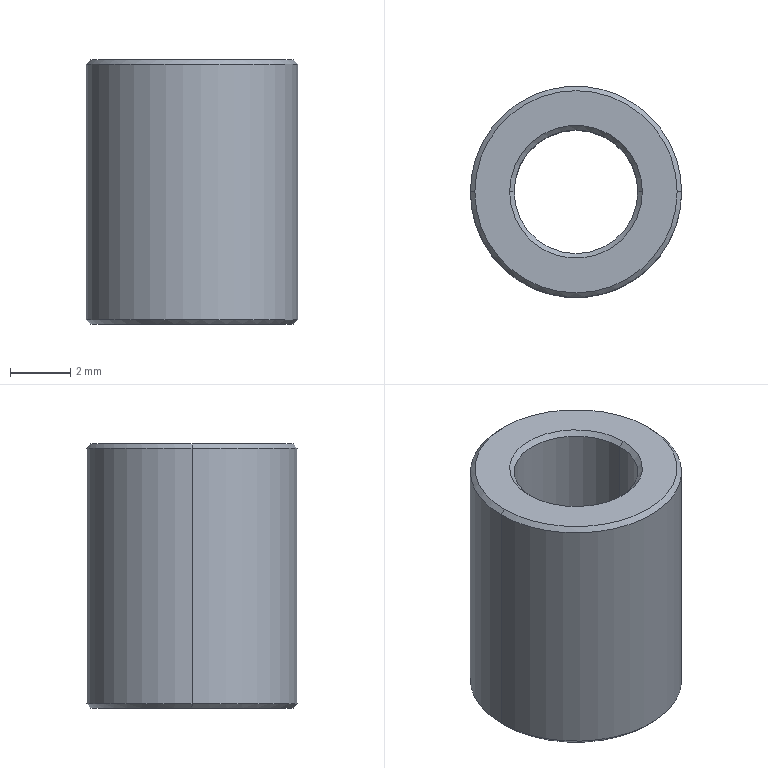Part | NX | features BREP 1 | 1 solid | 14 faces | box 7 x 7 x 8.75 mm | volume 220.433 mm3 | cone 8 | cylinder 4 | plane 2 | commonest cylinder face diameters 4.1 x2 7 x2
STEP:
#1=CARTESIAN_POINT('',(3.35,0.,8.75));
#2=VERTEX_POINT('',#1);
#3=CARTESIAN_POINT('',(3.5,0.,8.6));
#4=VERTEX_POINT('',#3);
#5=CARTESIAN_POINT('',(3.35,0.,8.75));
#6=DIRECTION('',(0.7071,0.,-0.7071));
#7=VECTOR('',#6,1000.);
#8=LINE('',#5,#7);
#9=EDGE_CURVE('',#2,#4,#8,.T.);
#10=ORIENTED_EDGE('',*,*,#9,.F.);
#11=CARTESIAN_POINT('',(-3.35,0.,8.75));
#12=VERTEX_POINT('',#11);
#13=CARTESIAN_POINT('',(0.,0.,8.75));
#14=DIRECTION('',(0.,0.,1.));
#15=DIRECTION('',(1.,0.,0.));
#16=AXIS2_PLACEMENT_3D('',#13,#14,#15);
#17=CIRCLE('',#16,3.35);
#18=EDGE_CURVE('',#12,#2,#17,.T.);
#19=ORIENTED_EDGE('',*,*,#18,.F.);
#20=CARTESIAN_POINT('',(-3.5,0.,8.6));
#21=VERTEX_POINT('',#20);
#22=CARTESIAN_POINT('',(-3.35,0.,8.75));
#23=DIRECTION('',(-0.7071,0.,-0.7071));
#24=VECTOR('',#23,1000.);
#25=LINE('',#22,#24);
#26=EDGE_CURVE('',#12,#21,#25,.T.);
#27=ORIENTED_EDGE('',*,*,#26,.T.);
#28=CARTESIAN_POINT('',(0.,0.,8.6));
#29=DIRECTION('',(0.,0.,-1.));
#30=DIRECTION('',(1.,0.,0.));
#31=AXIS2_PLACEMENT_3D('',#28,#29,#30);
#32=CIRCLE('',#31,3.5);
#33=EDGE_CURVE('',#4,#21,#32,.T.);
#34=ORIENTED_EDGE('',*,*,#33,.F.);
#35=EDGE_LOOP('',(#10,#19,#27,#34));
#36=FACE_BOUND('',#35,.T.);
#37=CARTESIAN_POINT('',(0.,0.,8.75));
#38=DIRECTION('',(0.,0.,-1.));
#39=DIRECTION('',(-1.,0.,0.));
#40=AXIS2_PLACEMENT_3D('',#37,#38,#39);
#41=CONICAL_SURFACE('',#40,3.35,0.7854);
#42=ADVANCED_FACE('',(#36),#41,.T.);
#43=CARTESIAN_POINT('',(-2.2,0.,8.75));
#44=VERTEX_POINT('',#43);
#45=CARTESIAN_POINT('',(-2.05,0.,8.6));
#46=VERTEX_POINT('',#45);
#47=CARTESIAN_POINT('',(-2.05,0.,8.6));
#48=DIRECTION('',(-0.7071,0.,0.7071));
#49=VECTOR('',#48,1000.);
#50=LINE('',#47,#49);
#51=EDGE_CURVE('',#44,#46,#50,.F.);
#52=ORIENTED_EDGE('',*,*,#51,.T.);
#53=CARTESIAN_POINT('',(2.05,0.,8.6));
#54=VERTEX_POINT('',#53);
#55=CARTESIAN_POINT('',(0.,0.,8.6));
#56=DIRECTION('',(0.,0.,1.));
#57=DIRECTION('',(1.,0.,0.));
#58=AXIS2_PLACEMENT_3D('',#55,#56,#57);
#59=CIRCLE('',#58,2.05);
#60=EDGE_CURVE('',#54,#46,#59,.T.);
#61=ORIENTED_EDGE('',*,*,#60,.F.);
#62=CARTESIAN_POINT('',(2.2,0.,8.75));
#63=VERTEX_POINT('',#62);
#64=CARTESIAN_POINT('',(2.05,0.,8.6));
#65=DIRECTION('',(0.7071,0.,0.7071));
#66=VECTOR('',#65,1000.);
#67=LINE('',#64,#66);
#68=EDGE_CURVE('',#63,#54,#67,.F.);
#69=ORIENTED_EDGE('',*,*,#68,.F.);
#70=CARTESIAN_POINT('',(0.,0.,8.75));
#71=DIRECTION('',(0.,0.,-1.));
#72=DIRECTION('',(1.,0.,0.));
#73=AXIS2_PLACEMENT_3D('',#70,#71,#72);
#74=CIRCLE('',#73,2.2);
#75=EDGE_CURVE('',#44,#63,#74,.T.);
#76=ORIENTED_EDGE('',*,*,#75,.F.);
#77=EDGE_LOOP('',(#52,#61,#69,#76));
#78=FACE_BOUND('',#77,.T.);
#79=CARTESIAN_POINT('',(0.,0.,8.6));
#80=DIRECTION('',(0.,0.,1.));
#81=DIRECTION('',(1.,0.,0.));
#82=AXIS2_PLACEMENT_3D('',#79,#80,#81);
#83=CONICAL_SURFACE('',#82,2.05,0.7854);
#84=ADVANCED_FACE('',(#78),#83,.F.);
#85=CARTESIAN_POINT('',(-3.5,0.,0.15));
#86=VERTEX_POINT('',#85);
#87=CARTESIAN_POINT('',(-3.35,0.,0.));
#88=VERTEX_POINT('',#87);
#89=CARTESIAN_POINT('',(-3.5,0.,0.15));
#90=DIRECTION('',(-0.7071,0.,0.7071));
#91=VECTOR('',#90,1000.);
#92=LINE('',#89,#91);
#93=EDGE_CURVE('',#86,#88,#92,.F.);
#94=ORIENTED_EDGE('',*,*,#93,.T.);
#95=CARTESIAN_POINT('',(3.35,0.,0.));
#96=VERTEX_POINT('',#95);
#97=CARTESIAN_POINT('',(0.,0.,0.));
#98=DIRECTION('',(0.,0.,-1.));
#99=DIRECTION('',(1.,0.,0.));
#100=AXIS2_PLACEMENT_3D('',#97,#98,#99);
#101=CIRCLE('',#100,3.35);
#102=EDGE_CURVE('',#96,#88,#101,.T.);
#103=ORIENTED_EDGE('',*,*,#102,.F.);
#104=CARTESIAN_POINT('',(3.5,0.,0.15));
#105=VERTEX_POINT('',#104);
#106=CARTESIAN_POINT('',(3.5,0.,0.15));
#107=DIRECTION('',(0.7071,0.,0.7071));
#108=VECTOR('',#107,1000.);
#109=LINE('',#106,#108);
#110=EDGE_CURVE('',#105,#96,#109,.F.);
#111=ORIENTED_EDGE('',*,*,#110,.F.);
#112=CARTESIAN_POINT('',(0.,0.,0.15));
#113=DIRECTION('',(0.,0.,1.));
#114=DIRECTION('',(1.,0.,0.));
#115=AXIS2_PLACEMENT_3D('',#112,#113,#114);
#116=CIRCLE('',#115,3.5);
#117=EDGE_CURVE('',#86,#105,#116,.T.);
#118=ORIENTED_EDGE('',*,*,#117,.F.);
#119=EDGE_LOOP('',(#94,#103,#111,#118));
#120=FACE_BOUND('',#119,.T.);
#121=CARTESIAN_POINT('',(0.,0.,0.15));
#122=DIRECTION('',(0.,0.,1.));
#123=DIRECTION('',(1.,0.,0.));
#124=AXIS2_PLACEMENT_3D('',#121,#122,#123);
#125=CONICAL_SURFACE('',#124,3.5,0.7854);
#126=ADVANCED_FACE('',(#120),#125,.T.);
#127=CARTESIAN_POINT('',(2.05,0.,0.15));
#128=VERTEX_POINT('',#127);
#129=CARTESIAN_POINT('',(2.2,0.,0.));
#130=VERTEX_POINT('',#129);
#131=CARTESIAN_POINT('',(2.2,0.,0.));
#132=DIRECTION('',(0.7071,0.,-0.7071));
#133=VECTOR('',#132,1000.);
#134=LINE('',#131,#133);
#135=EDGE_CURVE('',#128,#130,#134,.T.);
#136=ORIENTED_EDGE('',*,*,#135,.F.);
#137=CARTESIAN_POINT('',(-2.05,0.,0.15));
#138=VERTEX_POINT('',#137);
#139=CARTESIAN_POINT('',(0.,0.,0.15));
#140=DIRECTION('',(0.,0.,-1.));
#141=DIRECTION('',(1.,0.,0.));
#142=AXIS2_PLACEMENT_3D('',#139,#140,#141);
#143=CIRCLE('',#142,2.05);
#144=EDGE_CURVE('',#138,#128,#143,.T.);
#145=ORIENTED_EDGE('',*,*,#144,.F.);
#146=CARTESIAN_POINT('',(-2.2,0.,0.));
#147=VERTEX_POINT('',#146);
#148=CARTESIAN_POINT('',(-2.2,0.,0.));
#149=DIRECTION('',(-0.7071,0.,-0.7071));
#150=VECTOR('',#149,1000.);
#151=LINE('',#148,#150);
#152=EDGE_CURVE('',#138,#147,#151,.T.);
#153=ORIENTED_EDGE('',*,*,#152,.T.);
#154=CARTESIAN_POINT('',(0.,0.,0.));
#155=DIRECTION('',(0.,0.,1.));
#156=DIRECTION('',(1.,0.,0.));
#157=AXIS2_PLACEMENT_3D('',#154,#155,#156);
#158=CIRCLE('',#157,2.2);
#159=EDGE_CURVE('',#130,#147,#158,.T.);
#160=ORIENTED_EDGE('',*,*,#159,.F.);
#161=EDGE_LOOP('',(#136,#145,#153,#160));
#162=FACE_BOUND('',#161,.T.);
#163=CARTESIAN_POINT('',(0.,0.,0.));
#164=DIRECTION('',(0.,0.,-1.));
#165=DIRECTION('',(-1.,0.,0.));
#166=AXIS2_PLACEMENT_3D('',#163,#164,#165);
#167=CONICAL_SURFACE('',#166,2.2,0.7854);
#168=ADVANCED_FACE('',(#162),#167,.F.);
#169=CARTESIAN_POINT('',(2.05,0.,8.75));
#170=DIRECTION('',(0.,0.,-1.));
#171=VECTOR('',#170,1000.);
#172=LINE('',#169,#171);
#173=EDGE_CURVE('',#54,#128,#172,.T.);
#174=ORIENTED_EDGE('',*,*,#173,.F.);
#175=ORIENTED_EDGE('',*,*,#60,.T.);
#176=CARTESIAN_POINT('',(-2.05,0.,8.75));
#177=DIRECTION('',(0.,0.,-1.));
#178=VECTOR('',#177,1000.);
#179=LINE('',#176,#178);
#180=EDGE_CURVE('',#46,#138,#179,.T.);
#181=ORIENTED_EDGE('',*,*,#180,.T.);
#182=ORIENTED_EDGE('',*,*,#144,.T.);
#183=EDGE_LOOP('',(#174,#175,#181,#182));
#184=FACE_BOUND('',#183,.T.);
#185=CARTESIAN_POINT('',(0.,0.,8.75));
#186=DIRECTION('',(0.,0.,-1.));
#187=DIRECTION('',(-1.,0.,0.));
#188=AXIS2_PLACEMENT_3D('',#185,#186,#187);
#189=CYLINDRICAL_SURFACE('',#188,2.05);
#190=ADVANCED_FACE('',(#184),#189,.F.);
#191=CARTESIAN_POINT('',(3.5,0.,8.75));
#192=DIRECTION('',(0.,0.,-1.));
#193=VECTOR('',#192,1000.);
#194=LINE('',#191,#193);
#195=EDGE_CURVE('',#4,#105,#194,.T.);
#196=ORIENTED_EDGE('',*,*,#195,.F.);
#197=ORIENTED_EDGE('',*,*,#33,.T.);
#198=CARTESIAN_POINT('',(-3.5,0.,8.75));
#199=DIRECTION('',(0.,0.,-1.));
#200=VECTOR('',#199,1000.);
#201=LINE('',#198,#200);
#202=EDGE_CURVE('',#21,#86,#201,.T.);
#203=ORIENTED_EDGE('',*,*,#202,.T.);
#204=ORIENTED_EDGE('',*,*,#117,.T.);
#205=EDGE_LOOP('',(#196,#197,#203,#204));
#206=FACE_BOUND('',#205,.T.);
#207=CARTESIAN_POINT('',(0.,0.,8.75));
#208=DIRECTION('',(0.,0.,-1.));
#209=DIRECTION('',(-1.,0.,0.));
#210=AXIS2_PLACEMENT_3D('',#207,#208,#209);
#211=CYLINDRICAL_SURFACE('',#210,3.5);
#212=ADVANCED_FACE('',(#206),#211,.T.);
#213=ORIENTED_EDGE('',*,*,#102,.T.);
#214=CARTESIAN_POINT('',(0.,0.,0.));
#215=DIRECTION('',(0.,0.,-1.));
#216=DIRECTION('',(1.,0.,0.));
#217=AXIS2_PLACEMENT_3D('',#214,#215,#216);
#218=CIRCLE('',#217,3.35);
#219=EDGE_CURVE('',#88,#96,#218,.T.);
#220=ORIENTED_EDGE('',*,*,#219,.T.);
#221=EDGE_LOOP('',(#213,#220));
#222=FACE_BOUND('',#221,.T.);
#223=CARTESIAN_POINT('',(0.,0.,0.));
#224=DIRECTION('',(0.,0.,1.));
#225=DIRECTION('',(1.,0.,0.));
#226=AXIS2_PLACEMENT_3D('',#223,#224,#225);
#227=CIRCLE('',#226,2.2);
#228=EDGE_CURVE('',#147,#130,#227,.T.);
#229=ORIENTED_EDGE('',*,*,#228,.T.);
#230=ORIENTED_EDGE('',*,*,#159,.T.);
#231=EDGE_LOOP('',(#229,#230));
#232=FACE_BOUND('',#231,.T.);
#233=CARTESIAN_POINT('',(0.,0.,0.));
#234=DIRECTION('',(0.,0.,1.));
#235=DIRECTION('',(1.,0.,0.));
#236=AXIS2_PLACEMENT_3D('',#233,#234,#235);
#237=PLANE('',#236);
#238=ADVANCED_FACE('',(#222,#232),#237,.F.);
#239=ORIENTED_EDGE('',*,*,#18,.T.);
#240=CARTESIAN_POINT('',(0.,0.,8.75));
#241=DIRECTION('',(0.,0.,1.));
#242=DIRECTION('',(1.,0.,0.));
#243=AXIS2_PLACEMENT_3D('',#240,#241,#242);
#244=CIRCLE('',#243,3.35);
#245=EDGE_CURVE('',#2,#12,#244,.T.);
#246=ORIENTED_EDGE('',*,*,#245,.T.);
#247=EDGE_LOOP('',(#239,#246));
#248=FACE_BOUND('',#247,.T.);
#249=CARTESIAN_POINT('',(0.,0.,8.75));
#250=DIRECTION('',(0.,0.,-1.));
#251=DIRECTION('',(1.,0.,0.));
#252=AXIS2_PLACEMENT_3D('',#249,#250,#251);
#253=CIRCLE('',#252,2.2);
#254=EDGE_CURVE('',#63,#44,#253,.T.);
#255=ORIENTED_EDGE('',*,*,#254,.T.);
#256=ORIENTED_EDGE('',*,*,#75,.T.);
#257=EDGE_LOOP('',(#255,#256));
#258=FACE_BOUND('',#257,.T.);
#259=CARTESIAN_POINT('',(0.,0.,8.75));
#260=DIRECTION('',(0.,0.,1.));
#261=DIRECTION('',(1.,0.,0.));
#262=AXIS2_PLACEMENT_3D('',#259,#260,#261);
#263=PLANE('',#262);
#264=ADVANCED_FACE('',(#248,#258),#263,.T.);
#265=CARTESIAN_POINT('',(0.,0.,8.6));
#266=DIRECTION('',(0.,0.,-1.));
#267=DIRECTION('',(1.,0.,0.));
#268=AXIS2_PLACEMENT_3D('',#265,#266,#267);
#269=CIRCLE('',#268,3.5);
#270=EDGE_CURVE('',#21,#4,#269,.T.);
#271=ORIENTED_EDGE('',*,*,#270,.T.);
#272=ORIENTED_EDGE('',*,*,#195,.T.);
#273=CARTESIAN_POINT('',(0.,0.,0.15));
#274=DIRECTION('',(0.,0.,1.));
#275=DIRECTION('',(1.,0.,0.));
#276=AXIS2_PLACEMENT_3D('',#273,#274,#275);
#277=CIRCLE('',#276,3.5);
#278=EDGE_CURVE('',#105,#86,#277,.T.);
#279=ORIENTED_EDGE('',*,*,#278,.T.);
#280=ORIENTED_EDGE('',*,*,#202,.F.);
#281=EDGE_LOOP('',(#271,#272,#279,#280));
#282=FACE_BOUND('',#281,.T.);
#283=CARTESIAN_POINT('',(0.,0.,8.75));
#284=DIRECTION('',(0.,0.,-1.));
#285=DIRECTION('',(-1.,0.,0.));
#286=AXIS2_PLACEMENT_3D('',#283,#284,#285);
#287=CYLINDRICAL_SURFACE('',#286,3.5);
#288=ADVANCED_FACE('',(#282),#287,.T.);
#289=CARTESIAN_POINT('',(0.,0.,8.6));
#290=DIRECTION('',(0.,0.,1.));
#291=DIRECTION('',(1.,0.,0.));
#292=AXIS2_PLACEMENT_3D('',#289,#290,#291);
#293=CIRCLE('',#292,2.05);
#294=EDGE_CURVE('',#46,#54,#293,.T.);
#295=ORIENTED_EDGE('',*,*,#294,.T.);
#296=ORIENTED_EDGE('',*,*,#173,.T.);
#297=CARTESIAN_POINT('',(0.,0.,0.15));
#298=DIRECTION('',(0.,0.,-1.));
#299=DIRECTION('',(1.,0.,0.));
#300=AXIS2_PLACEMENT_3D('',#297,#298,#299);
#301=CIRCLE('',#300,2.05);
#302=EDGE_CURVE('',#128,#138,#301,.T.);
#303=ORIENTED_EDGE('',*,*,#302,.T.);
#304=ORIENTED_EDGE('',*,*,#180,.F.);
#305=EDGE_LOOP('',(#295,#296,#303,#304));
#306=FACE_BOUND('',#305,.T.);
#307=CARTESIAN_POINT('',(0.,0.,8.75));
#308=DIRECTION('',(0.,0.,-1.));
#309=DIRECTION('',(-1.,0.,0.));
#310=AXIS2_PLACEMENT_3D('',#307,#308,#309);
#311=CYLINDRICAL_SURFACE('',#310,2.05);
#312=ADVANCED_FACE('',(#306),#311,.F.);
#313=ORIENTED_EDGE('',*,*,#302,.F.);
#314=ORIENTED_EDGE('',*,*,#135,.T.);
#315=ORIENTED_EDGE('',*,*,#228,.F.);
#316=ORIENTED_EDGE('',*,*,#152,.F.);
#317=EDGE_LOOP('',(#313,#314,#315,#316));
#318=FACE_BOUND('',#317,.T.);
#319=CARTESIAN_POINT('',(0.,0.,0.));
#320=DIRECTION('',(0.,0.,-1.));
#321=DIRECTION('',(-1.,0.,0.));
#322=AXIS2_PLACEMENT_3D('',#319,#320,#321);
#323=CONICAL_SURFACE('',#322,2.2,0.7854);
#324=ADVANCED_FACE('',(#318),#323,.F.);
#325=ORIENTED_EDGE('',*,*,#219,.F.);
#326=ORIENTED_EDGE('',*,*,#93,.F.);
#327=ORIENTED_EDGE('',*,*,#278,.F.);
#328=ORIENTED_EDGE('',*,*,#110,.T.);
#329=EDGE_LOOP('',(#325,#326,#327,#328));
#330=FACE_BOUND('',#329,.T.);
#331=CARTESIAN_POINT('',(0.,0.,0.15));
#332=DIRECTION('',(0.,0.,1.));
#333=DIRECTION('',(1.,0.,0.));
#334=AXIS2_PLACEMENT_3D('',#331,#332,#333);
#335=CONICAL_SURFACE('',#334,3.5,0.7854);
#336=ADVANCED_FACE('',(#330),#335,.T.);
#337=ORIENTED_EDGE('',*,*,#294,.F.);
#338=ORIENTED_EDGE('',*,*,#51,.F.);
#339=ORIENTED_EDGE('',*,*,#254,.F.);
#340=ORIENTED_EDGE('',*,*,#68,.T.);
#341=EDGE_LOOP('',(#337,#338,#339,#340));
#342=FACE_BOUND('',#341,.T.);
#343=CARTESIAN_POINT('',(0.,0.,8.6));
#344=DIRECTION('',(0.,0.,1.));
#345=DIRECTION('',(1.,0.,0.));
#346=AXIS2_PLACEMENT_3D('',#343,#344,#345);
#347=CONICAL_SURFACE('',#346,2.05,0.7854);
#348=ADVANCED_FACE('',(#342),#347,.F.);
#349=ORIENTED_EDGE('',*,*,#245,.F.);
#350=ORIENTED_EDGE('',*,*,#9,.T.);
#351=ORIENTED_EDGE('',*,*,#270,.F.);
#352=ORIENTED_EDGE('',*,*,#26,.F.);
#353=EDGE_LOOP('',(#349,#350,#351,#352));
#354=FACE_BOUND('',#353,.T.);
#355=CARTESIAN_POINT('',(0.,0.,8.75));
#356=DIRECTION('',(0.,0.,-1.));
#357=DIRECTION('',(-1.,0.,0.));
#358=AXIS2_PLACEMENT_3D('',#355,#356,#357);
#359=CONICAL_SURFACE('',#358,3.35,0.7854);
#360=ADVANCED_FACE('',(#354),#359,.T.);
#361=CLOSED_SHELL('',(#42,#84,#126,#168,#190,#212,#238,#264,#288,#312,#324,#336,#348,#360));
#362=MANIFOLD_SOLID_BREP('',#361);
#363=(LENGTH_UNIT()NAMED_UNIT(*)SI_UNIT(.MILLI.,.METRE.));
#364=UNCERTAINTY_MEASURE_WITH_UNIT(LENGTH_MEASURE(0.00001),#363,'','');
#365=(NAMED_UNIT(*)PLANE_ANGLE_UNIT()SI_UNIT($,.RADIAN.));
#366=(NAMED_UNIT(*)SI_UNIT($,.STERADIAN.)SOLID_ANGLE_UNIT());
#367=(GEOMETRIC_REPRESENTATION_CONTEXT(3)GLOBAL_UNCERTAINTY_ASSIGNED_CONTEXT((#364))GLOBAL_UNIT_ASSIGNED_CONTEXT((#363,#365,#366))REPRESENTATION_CONTEXT('',''));
#368=ADVANCED_BREP_SHAPE_REPRESENTATION('',(#362),#367);